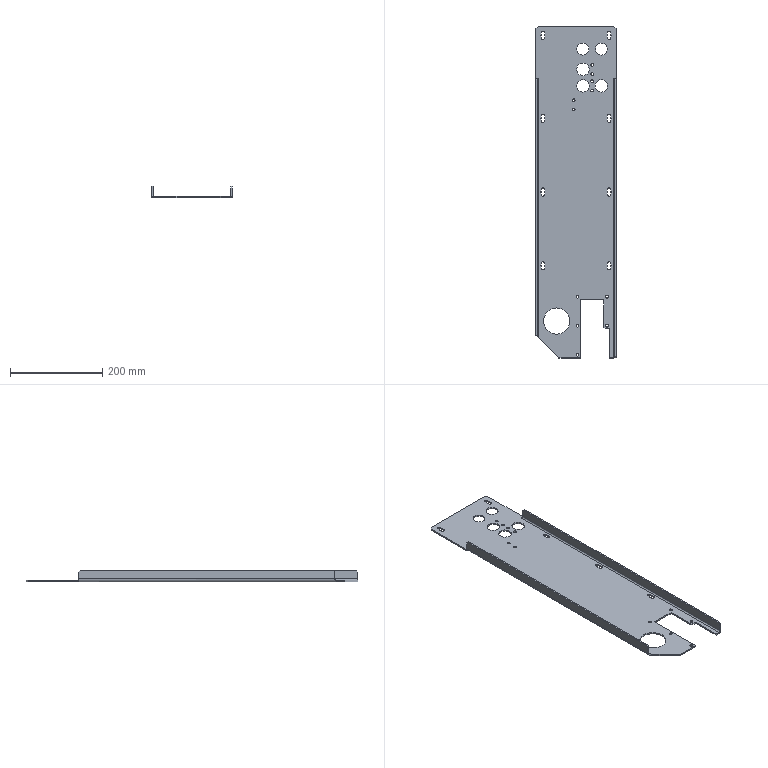Part | NX | features solid 2 | 1 solid | 143 faces | box 174 x 720 x 25 mm | volume 400796 mm3 | cylinder 78 | plane 64 | spline 1 | commonest cylinder face diameters 6 x24 7.5 x24 8 x16 27 x6 26 x4 12 x2